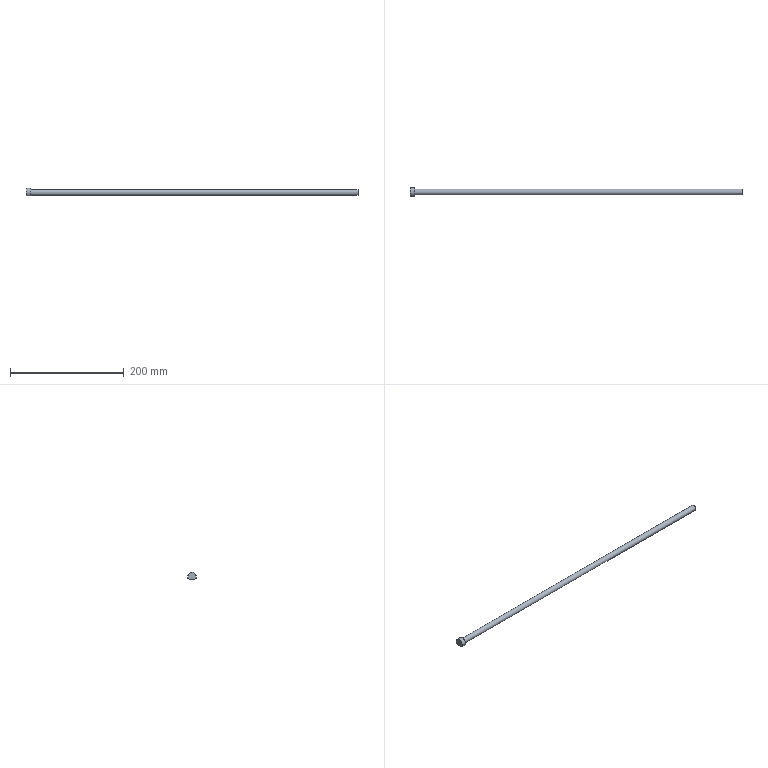Part | STEP file | solid 48 | 1 solid | 6 faces | box 585 x 15 x 13 mm | volume 46619 mm3 | plane 4 | cylinder 2 | commonest cylinder face diameters 10 x1 15 x1